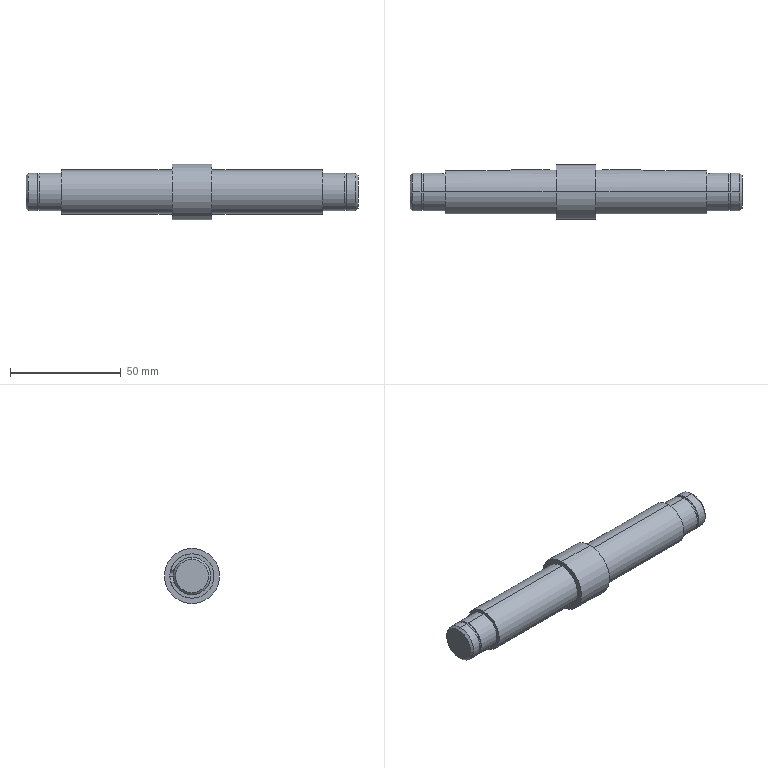Part | STEP file | CON-002 | 1 solid | 46 faces | box 150 x 25 x 25 mm | volume 46152 mm3 | cylinder 26 | plane 16 | cone 4 | commonest cylinder face diameters 6 x8 17 x8 16.2 x4 20 x4 25 x2